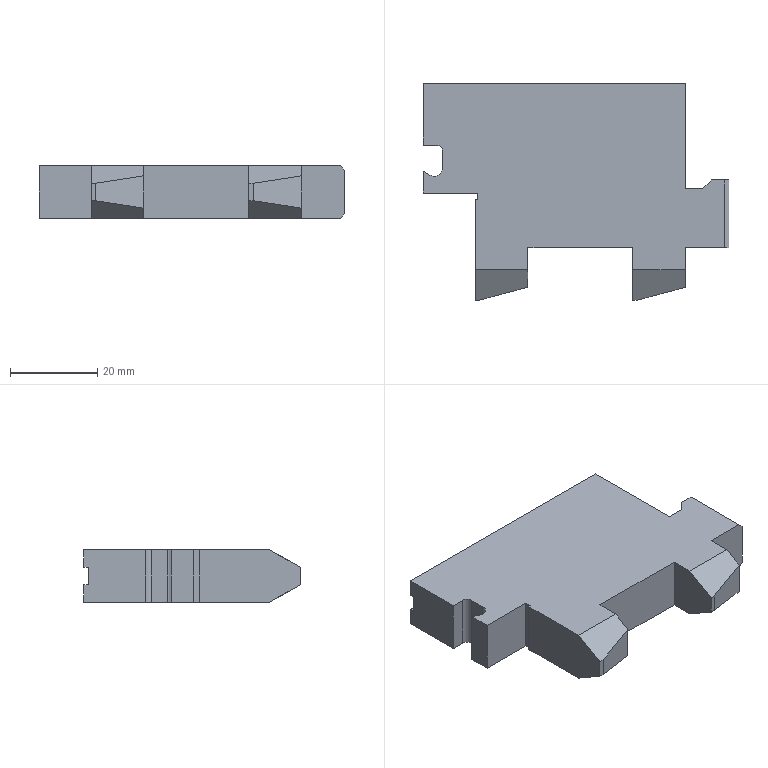Part | SolidWorks | features ICE 2, Chamfer 1, Extrusion 1 | 1 solid | 38 faces | box 70 x 49.5 x 12 mm | volume 28944 mm3 | plane 36 | cylinder 2 | commonest cylinder face diameters 3 x1 4 x1
STEP:
#1=CARTESIAN_POINT('',(0.,25.,-2.));
#2=VERTEX_POINT('',#1);
#3=CARTESIAN_POINT('',(0.,25.,-6.));
#4=VERTEX_POINT('',#3);
#5=CARTESIAN_POINT('',(0.,25.,6.));
#6=DIRECTION('',(0.,0.,-1.));
#7=VECTOR('',#6,1000.);
#8=LINE('',#5,#7);
#9=EDGE_CURVE('',#2,#4,#8,.T.);
#10=ORIENTED_EDGE('',*,*,#9,.F.);
#11=CARTESIAN_POINT('',(60.,25.,-2.));
#12=VERTEX_POINT('',#11);
#13=CARTESIAN_POINT('',(0.,25.,-2.));
#14=DIRECTION('',(-1.,0.,0.));
#15=VECTOR('',#14,1000.);
#16=LINE('',#13,#15);
#17=EDGE_CURVE('',#12,#2,#16,.T.);
#18=ORIENTED_EDGE('',*,*,#17,.F.);
#19=CARTESIAN_POINT('',(60.,25.,-6.));
#20=VERTEX_POINT('',#19);
#21=CARTESIAN_POINT('',(60.,25.,6.));
#22=DIRECTION('',(0.,0.,-1.));
#23=VECTOR('',#22,1000.);
#24=LINE('',#21,#23);
#25=EDGE_CURVE('',#12,#20,#24,.T.);
#26=ORIENTED_EDGE('',*,*,#25,.T.);
#27=CARTESIAN_POINT('',(0.,25.,-6.));
#28=DIRECTION('',(-1.,0.,0.));
#29=VECTOR('',#28,1000.);
#30=LINE('',#27,#29);
#31=EDGE_CURVE('',#20,#4,#30,.T.);
#32=ORIENTED_EDGE('',*,*,#31,.T.);
#33=EDGE_LOOP('',(#10,#18,#26,#32));
#34=FACE_OUTER_BOUND('',#33,.T.);
#35=CARTESIAN_POINT('',(0.,25.,6.));
#36=DIRECTION('',(0.,-1.,0.));
#37=DIRECTION('',(1.,0.,0.));
#38=AXIS2_PLACEMENT_3D('',#35,#36,#37);
#39=PLANE('',#38);
#40=ADVANCED_FACE('',(#34),#39,.F.);
#41=CARTESIAN_POINT('',(0.,0.,-6.));
#42=VERTEX_POINT('',#41);
#43=CARTESIAN_POINT('',(12.5,0.,-6.));
#44=VERTEX_POINT('',#43);
#45=CARTESIAN_POINT('',(12.5,0.,-6.));
#46=DIRECTION('',(1.,0.,0.));
#47=VECTOR('',#46,1000.);
#48=LINE('',#45,#47);
#49=EDGE_CURVE('',#42,#44,#48,.T.);
#50=ORIENTED_EDGE('',*,*,#49,.T.);
#51=CARTESIAN_POINT('',(12.5,0.,6.));
#52=VERTEX_POINT('',#51);
#53=CARTESIAN_POINT('',(12.5,0.,6.));
#54=DIRECTION('',(0.,0.,-1.));
#55=VECTOR('',#54,1000.);
#56=LINE('',#53,#55);
#57=EDGE_CURVE('',#52,#44,#56,.T.);
#58=ORIENTED_EDGE('',*,*,#57,.F.);
#59=CARTESIAN_POINT('',(0.,0.,6.));
#60=VERTEX_POINT('',#59);
#61=CARTESIAN_POINT('',(12.5,0.,6.));
#62=DIRECTION('',(1.,0.,0.));
#63=VECTOR('',#62,1000.);
#64=LINE('',#61,#63);
#65=EDGE_CURVE('',#60,#52,#64,.T.);
#66=ORIENTED_EDGE('',*,*,#65,.F.);
#67=CARTESIAN_POINT('',(0.,0.,6.));
#68=DIRECTION('',(0.,0.,-1.));
#69=VECTOR('',#68,1000.);
#70=LINE('',#67,#69);
#71=EDGE_CURVE('',#60,#42,#70,.T.);
#72=ORIENTED_EDGE('',*,*,#71,.T.);
#73=EDGE_LOOP('',(#50,#58,#66,#72));
#74=FACE_OUTER_BOUND('',#73,.T.);
#75=CARTESIAN_POINT('',(12.5,0.,6.));
#76=DIRECTION('',(0.,1.,0.));
#77=DIRECTION('',(-1.,0.,0.));
#78=AXIS2_PLACEMENT_3D('',#75,#76,#77);
#79=PLANE('',#78);
#80=ADVANCED_FACE('',(#74),#79,.F.);
#81=CARTESIAN_POINT('',(12.5,-1.5,-6.));
#82=VERTEX_POINT('',#81);
#83=CARTESIAN_POINT('',(12.5,0.,-6.));
#84=DIRECTION('',(0.,-1.,0.));
#85=VECTOR('',#84,1000.);
#86=LINE('',#83,#85);
#87=EDGE_CURVE('',#44,#82,#86,.T.);
#88=ORIENTED_EDGE('',*,*,#87,.T.);
#89=CARTESIAN_POINT('',(12.5,-1.5,6.));
#90=VERTEX_POINT('',#89);
#91=CARTESIAN_POINT('',(12.5,-1.5,6.));
#92=DIRECTION('',(0.,0.,-1.));
#93=VECTOR('',#92,1000.);
#94=LINE('',#91,#93);
#95=EDGE_CURVE('',#90,#82,#94,.T.);
#96=ORIENTED_EDGE('',*,*,#95,.F.);
#97=CARTESIAN_POINT('',(12.5,0.,6.));
#98=DIRECTION('',(0.,-1.,0.));
#99=VECTOR('',#98,1000.);
#100=LINE('',#97,#99);
#101=EDGE_CURVE('',#52,#90,#100,.T.);
#102=ORIENTED_EDGE('',*,*,#101,.F.);
#103=ORIENTED_EDGE('',*,*,#57,.T.);
#104=EDGE_LOOP('',(#88,#96,#102,#103));
#105=FACE_OUTER_BOUND('',#104,.T.);
#106=CARTESIAN_POINT('',(12.5,0.,6.));
#107=DIRECTION('',(1.,0.,0.));
#108=DIRECTION('',(0.,0.,-1.));
#109=AXIS2_PLACEMENT_3D('',#106,#107,#108);
#110=PLANE('',#109);
#111=ADVANCED_FACE('',(#105),#110,.F.);
#112=CARTESIAN_POINT('',(12.,-1.5,-6.));
#113=VERTEX_POINT('',#112);
#114=CARTESIAN_POINT('',(12.5,-1.5,-6.));
#115=DIRECTION('',(-1.,0.,0.));
#116=VECTOR('',#115,1000.);
#117=LINE('',#114,#116);
#118=EDGE_CURVE('',#82,#113,#117,.T.);
#119=ORIENTED_EDGE('',*,*,#118,.T.);
#120=CARTESIAN_POINT('',(12.,-1.5,6.));
#121=VERTEX_POINT('',#120);
#122=CARTESIAN_POINT('',(12.,-1.5,6.));
#123=DIRECTION('',(0.,0.,-1.));
#124=VECTOR('',#123,1000.);
#125=LINE('',#122,#124);
#126=EDGE_CURVE('',#121,#113,#125,.T.);
#127=ORIENTED_EDGE('',*,*,#126,.F.);
#128=CARTESIAN_POINT('',(12.5,-1.5,6.));
#129=DIRECTION('',(-1.,0.,0.));
#130=VECTOR('',#129,1000.);
#131=LINE('',#128,#130);
#132=EDGE_CURVE('',#90,#121,#131,.T.);
#133=ORIENTED_EDGE('',*,*,#132,.F.);
#134=ORIENTED_EDGE('',*,*,#95,.T.);
#135=EDGE_LOOP('',(#119,#127,#133,#134));
#136=FACE_OUTER_BOUND('',#135,.T.);
#137=CARTESIAN_POINT('',(12.5,-1.5,6.));
#138=DIRECTION('',(0.,-1.,0.));
#139=DIRECTION('',(0.,0.,-1.));
#140=AXIS2_PLACEMENT_3D('',#137,#138,#139);
#141=PLANE('',#140);
#142=ADVANCED_FACE('',(#136),#141,.F.);
#143=CARTESIAN_POINT('',(12.,-17.572,-6.));
#144=VERTEX_POINT('',#143);
#145=CARTESIAN_POINT('',(12.,-1.5,-6.));
#146=DIRECTION('',(0.,-1.,0.));
#147=VECTOR('',#146,1000.);
#148=LINE('',#145,#147);
#149=EDGE_CURVE('',#113,#144,#148,.T.);
#150=ORIENTED_EDGE('',*,*,#149,.T.);
#151=CARTESIAN_POINT('',(12.,-24.5,-2.));
#152=VERTEX_POINT('',#151);
#153=CARTESIAN_POINT('',(12.,-24.5,-2.));
#154=DIRECTION('',(0.,0.866,-0.5));
#155=VECTOR('',#154,1000.);
#156=LINE('',#153,#155);
#157=EDGE_CURVE('',#152,#144,#156,.T.);
#158=ORIENTED_EDGE('',*,*,#157,.F.);
#159=CARTESIAN_POINT('',(12.,-24.5,2.));
#160=VERTEX_POINT('',#159);
#161=CARTESIAN_POINT('',(12.,-24.5,6.));
#162=DIRECTION('',(0.,0.,-1.));
#163=VECTOR('',#162,1000.);
#164=LINE('',#161,#163);
#165=EDGE_CURVE('',#160,#152,#164,.T.);
#166=ORIENTED_EDGE('',*,*,#165,.F.);
#167=CARTESIAN_POINT('',(12.,-17.572,6.));
#168=VERTEX_POINT('',#167);
#169=CARTESIAN_POINT('',(12.,-24.5,2.));
#170=DIRECTION('',(0.,-0.866,-0.5));
#171=VECTOR('',#170,1000.);
#172=LINE('',#169,#171);
#173=EDGE_CURVE('',#168,#160,#172,.T.);
#174=ORIENTED_EDGE('',*,*,#173,.F.);
#175=CARTESIAN_POINT('',(12.,-1.5,6.));
#176=DIRECTION('',(0.,-1.,0.));
#177=VECTOR('',#176,1000.);
#178=LINE('',#175,#177);
#179=EDGE_CURVE('',#121,#168,#178,.T.);
#180=ORIENTED_EDGE('',*,*,#179,.F.);
#181=ORIENTED_EDGE('',*,*,#126,.T.);
#182=EDGE_LOOP('',(#150,#158,#166,#174,#180,#181));
#183=FACE_OUTER_BOUND('',#182,.T.);
#184=CARTESIAN_POINT('',(12.,-1.5,6.));
#185=DIRECTION('',(1.,0.,0.));
#186=DIRECTION('',(0.,1.,0.));
#187=AXIS2_PLACEMENT_3D('',#184,#185,#186);
#188=PLANE('',#187);
#189=ADVANCED_FACE('',(#183),#188,.F.);
#190=ORIENTED_EDGE('',*,*,#165,.T.);
#191=CARTESIAN_POINT('',(13.,-24.5,-2.));
#192=VERTEX_POINT('',#191);
#193=CARTESIAN_POINT('',(70.,-24.5,-2.));
#194=DIRECTION('',(-1.,0.,0.));
#195=VECTOR('',#194,1000.);
#196=LINE('',#193,#195);
#197=EDGE_CURVE('',#192,#152,#196,.T.);
#198=ORIENTED_EDGE('',*,*,#197,.F.);
#199=CARTESIAN_POINT('',(13.,-24.5,2.));
#200=VERTEX_POINT('',#199);
#201=CARTESIAN_POINT('',(13.,-24.5,6.));
#202=DIRECTION('',(0.,0.,-1.));
#203=VECTOR('',#202,1000.);
#204=LINE('',#201,#203);
#205=EDGE_CURVE('',#200,#192,#204,.T.);
#206=ORIENTED_EDGE('',*,*,#205,.F.);
#207=CARTESIAN_POINT('',(70.,-24.5,2.));
#208=DIRECTION('',(-1.,0.,0.));
#209=VECTOR('',#208,1000.);
#210=LINE('',#207,#209);
#211=EDGE_CURVE('',#200,#160,#210,.T.);
#212=ORIENTED_EDGE('',*,*,#211,.T.);
#213=EDGE_LOOP('',(#190,#198,#206,#212));
#214=FACE_OUTER_BOUND('',#213,.T.);
#215=CARTESIAN_POINT('',(13.,-24.5,6.));
#216=DIRECTION('',(0.,1.,0.));
#217=DIRECTION('',(0.,0.,1.));
#218=AXIS2_PLACEMENT_3D('',#215,#216,#217);
#219=PLANE('',#218);
#220=ADVANCED_FACE('',(#214),#219,.F.);
#221=ORIENTED_EDGE('',*,*,#205,.T.);
#222=CARTESIAN_POINT('',(24.,-21.553,-3.702));
#223=VERTEX_POINT('',#222);
#224=CARTESIAN_POINT('',(22.63,-21.92,-3.49));
#225=DIRECTION('',(0.9553,0.256,-0.1478));
#226=VECTOR('',#225,1000.);
#227=LINE('',#224,#226);
#228=EDGE_CURVE('',#192,#223,#227,.T.);
#229=ORIENTED_EDGE('',*,*,#228,.T.);
#230=CARTESIAN_POINT('',(24.,-21.553,3.702));
#231=VERTEX_POINT('',#230);
#232=CARTESIAN_POINT('',(24.,-21.553,6.));
#233=DIRECTION('',(0.,0.,-1.));
#234=VECTOR('',#233,1000.);
#235=LINE('',#232,#234);
#236=EDGE_CURVE('',#231,#223,#235,.T.);
#237=ORIENTED_EDGE('',*,*,#236,.F.);
#238=CARTESIAN_POINT('',(24.324,-21.466,3.752));
#239=DIRECTION('',(-0.9553,-0.256,-0.1478));
#240=VECTOR('',#239,1000.);
#241=LINE('',#238,#240);
#242=EDGE_CURVE('',#231,#200,#241,.T.);
#243=ORIENTED_EDGE('',*,*,#242,.T.);
#244=EDGE_LOOP('',(#221,#229,#237,#243));
#245=FACE_OUTER_BOUND('',#244,.T.);
#246=CARTESIAN_POINT('',(24.,-21.553,6.));
#247=DIRECTION('',(-0.2588,0.9659,0.));
#248=DIRECTION('',(-0.9659,-0.2588,0.));
#249=AXIS2_PLACEMENT_3D('',#246,#247,#248);
#250=PLANE('',#249);
#251=ADVANCED_FACE('',(#245),#250,.F.);
#252=ORIENTED_EDGE('',*,*,#236,.T.);
#253=CARTESIAN_POINT('',(24.,-17.572,-6.));
#254=VERTEX_POINT('',#253);
#255=CARTESIAN_POINT('',(24.,-18.964,-5.196));
#256=DIRECTION('',(0.,0.866,-0.5));
#257=VECTOR('',#256,1000.);
#258=LINE('',#255,#257);
#259=EDGE_CURVE('',#223,#254,#258,.T.);
#260=ORIENTED_EDGE('',*,*,#259,.T.);
#261=CARTESIAN_POINT('',(24.,-12.5,-6.));
#262=VERTEX_POINT('',#261);
#263=CARTESIAN_POINT('',(24.,-12.5,-6.));
#264=DIRECTION('',(0.,1.,0.));
#265=VECTOR('',#264,1000.);
#266=LINE('',#263,#265);
#267=EDGE_CURVE('',#254,#262,#266,.T.);
#268=ORIENTED_EDGE('',*,*,#267,.T.);
#269=CARTESIAN_POINT('',(24.,-12.5,6.));
#270=VERTEX_POINT('',#269);
#271=CARTESIAN_POINT('',(24.,-12.5,6.));
#272=DIRECTION('',(0.,0.,-1.));
#273=VECTOR('',#272,1000.);
#274=LINE('',#271,#273);
#275=EDGE_CURVE('',#270,#262,#274,.T.);
#276=ORIENTED_EDGE('',*,*,#275,.F.);
#277=CARTESIAN_POINT('',(24.,-17.572,6.));
#278=VERTEX_POINT('',#277);
#279=CARTESIAN_POINT('',(24.,-12.5,6.));
#280=DIRECTION('',(0.,1.,0.));
#281=VECTOR('',#280,1000.);
#282=LINE('',#279,#281);
#283=EDGE_CURVE('',#278,#270,#282,.T.);
#284=ORIENTED_EDGE('',*,*,#283,.F.);
#285=CARTESIAN_POINT('',(24.,-13.768,8.196));
#286=DIRECTION('',(0.,-0.866,-0.5));
#287=VECTOR('',#286,1000.);
#288=LINE('',#285,#287);
#289=EDGE_CURVE('',#278,#231,#288,.T.);
#290=ORIENTED_EDGE('',*,*,#289,.T.);
#291=EDGE_LOOP('',(#252,#260,#268,#276,#284,#290));
#292=FACE_OUTER_BOUND('',#291,.T.);
#293=CARTESIAN_POINT('',(24.,-12.5,6.));
#294=DIRECTION('',(-1.,0.,0.));
#295=DIRECTION('',(0.,0.,1.));
#296=AXIS2_PLACEMENT_3D('',#293,#294,#295);
#297=PLANE('',#296);
#298=ADVANCED_FACE('',(#292),#297,.F.);
#299=CARTESIAN_POINT('',(48.,-12.5,-6.));
#300=VERTEX_POINT('',#299);
#301=CARTESIAN_POINT('',(48.,-12.5,-6.));
#302=DIRECTION('',(1.,0.,0.));
#303=VECTOR('',#302,1000.);
#304=LINE('',#301,#303);
#305=EDGE_CURVE('',#262,#300,#304,.T.);
#306=ORIENTED_EDGE('',*,*,#305,.T.);
#307=CARTESIAN_POINT('',(48.,-12.5,6.));
#308=VERTEX_POINT('',#307);
#309=CARTESIAN_POINT('',(48.,-12.5,6.));
#310=DIRECTION('',(0.,0.,-1.));
#311=VECTOR('',#310,1000.);
#312=LINE('',#309,#311);
#313=EDGE_CURVE('',#308,#300,#312,.T.);
#314=ORIENTED_EDGE('',*,*,#313,.F.);
#315=CARTESIAN_POINT('',(48.,-12.5,6.));
#316=DIRECTION('',(1.,0.,0.));
#317=VECTOR('',#316,1000.);
#318=LINE('',#315,#317);
#319=EDGE_CURVE('',#270,#308,#318,.T.);
#320=ORIENTED_EDGE('',*,*,#319,.F.);
#321=ORIENTED_EDGE('',*,*,#275,.T.);
#322=EDGE_LOOP('',(#306,#314,#320,#321));
#323=FACE_OUTER_BOUND('',#322,.T.);
#324=CARTESIAN_POINT('',(48.,-12.5,6.));
#325=DIRECTION('',(0.,1.,0.));
#326=DIRECTION('',(-1.,0.,0.));
#327=AXIS2_PLACEMENT_3D('',#324,#325,#326);
#328=PLANE('',#327);
#329=ADVANCED_FACE('',(#323),#328,.F.);
#330=CARTESIAN_POINT('',(48.,-17.572,-6.));
#331=VERTEX_POINT('',#330);
#332=CARTESIAN_POINT('',(48.,-24.5,-6.));
#333=DIRECTION('',(0.,-1.,0.));
#334=VECTOR('',#333,1000.);
#335=LINE('',#332,#334);
#336=EDGE_CURVE('',#300,#331,#335,.T.);
#337=ORIENTED_EDGE('',*,*,#336,.T.);
#338=CARTESIAN_POINT('',(48.,-24.5,-2.));
#339=VERTEX_POINT('',#338);
#340=CARTESIAN_POINT('',(48.,-27.964,0.));
#341=DIRECTION('',(0.,-0.866,0.5));
#342=VECTOR('',#341,1000.);
#343=LINE('',#340,#342);
#344=EDGE_CURVE('',#331,#339,#343,.T.);
#345=ORIENTED_EDGE('',*,*,#344,.T.);
#346=CARTESIAN_POINT('',(48.,-24.5,2.));
#347=VERTEX_POINT('',#346);
#348=CARTESIAN_POINT('',(48.,-24.5,6.));
#349=DIRECTION('',(0.,0.,-1.));
#350=VECTOR('',#349,1000.);
#351=LINE('',#348,#350);
#352=EDGE_CURVE('',#347,#339,#351,.T.);
#353=ORIENTED_EDGE('',*,*,#352,.F.);
#354=CARTESIAN_POINT('',(48.,-17.572,6.));
#355=VERTEX_POINT('',#354);
#356=CARTESIAN_POINT('',(48.,-22.768,3.));
#357=DIRECTION('',(0.,0.866,0.5));
#358=VECTOR('',#357,1000.);
#359=LINE('',#356,#358);
#360=EDGE_CURVE('',#347,#355,#359,.T.);
#361=ORIENTED_EDGE('',*,*,#360,.T.);
#362=CARTESIAN_POINT('',(48.,-24.5,6.));
#363=DIRECTION('',(0.,-1.,0.));
#364=VECTOR('',#363,1000.);
#365=LINE('',#362,#364);
#366=EDGE_CURVE('',#308,#355,#365,.T.);
#367=ORIENTED_EDGE('',*,*,#366,.F.);
#368=ORIENTED_EDGE('',*,*,#313,.T.);
#369=EDGE_LOOP('',(#337,#345,#353,#361,#367,#368));
#370=FACE_OUTER_BOUND('',#369,.T.);
#371=CARTESIAN_POINT('',(48.,-24.5,6.));
#372=DIRECTION('',(1.,0.,0.));
#373=DIRECTION('',(0.,0.,-1.));
#374=AXIS2_PLACEMENT_3D('',#371,#372,#373);
#375=PLANE('',#374);
#376=ADVANCED_FACE('',(#370),#375,.F.);
#377=ORIENTED_EDGE('',*,*,#352,.T.);
#378=CARTESIAN_POINT('',(49.,-24.5,-2.));
#379=VERTEX_POINT('',#378);
#380=CARTESIAN_POINT('',(70.,-24.5,-2.));
#381=DIRECTION('',(-1.,0.,0.));
#382=VECTOR('',#381,1000.);
#383=LINE('',#380,#382);
#384=EDGE_CURVE('',#379,#339,#383,.T.);
#385=ORIENTED_EDGE('',*,*,#384,.F.);
#386=CARTESIAN_POINT('',(49.,-24.5,2.));
#387=VERTEX_POINT('',#386);
#388=CARTESIAN_POINT('',(49.,-24.5,6.));
#389=DIRECTION('',(0.,0.,-1.));
#390=VECTOR('',#389,1000.);
#391=LINE('',#388,#390);
#392=EDGE_CURVE('',#387,#379,#391,.T.);
#393=ORIENTED_EDGE('',*,*,#392,.F.);
#394=CARTESIAN_POINT('',(70.,-24.5,2.));
#395=DIRECTION('',(-1.,0.,0.));
#396=VECTOR('',#395,1000.);
#397=LINE('',#394,#396);
#398=EDGE_CURVE('',#387,#347,#397,.T.);
#399=ORIENTED_EDGE('',*,*,#398,.T.);
#400=EDGE_LOOP('',(#377,#385,#393,#399));
#401=FACE_OUTER_BOUND('',#400,.T.);
#402=CARTESIAN_POINT('',(49.,-24.5,6.));
#403=DIRECTION('',(0.,1.,0.));
#404=DIRECTION('',(0.,0.,1.));
#405=AXIS2_PLACEMENT_3D('',#402,#403,#404);
#406=PLANE('',#405);
#407=ADVANCED_FACE('',(#401),#406,.F.);
#408=ORIENTED_EDGE('',*,*,#392,.T.);
#409=CARTESIAN_POINT('',(60.,-21.553,-3.702));
#410=VERTEX_POINT('',#409);
#411=CARTESIAN_POINT('',(58.63,-21.92,-3.49));
#412=DIRECTION('',(0.9553,0.256,-0.1478));
#413=VECTOR('',#412,1000.);
#414=LINE('',#411,#413);
#415=EDGE_CURVE('',#379,#410,#414,.T.);
#416=ORIENTED_EDGE('',*,*,#415,.T.);
#417=CARTESIAN_POINT('',(60.,-21.553,3.702));
#418=VERTEX_POINT('',#417);
#419=CARTESIAN_POINT('',(60.,-21.553,6.));
#420=DIRECTION('',(0.,0.,-1.));
#421=VECTOR('',#420,1000.);
#422=LINE('',#419,#421);
#423=EDGE_CURVE('',#418,#410,#422,.T.);
#424=ORIENTED_EDGE('',*,*,#423,.F.);
#425=CARTESIAN_POINT('',(60.324,-21.466,3.752));
#426=DIRECTION('',(-0.9553,-0.256,-0.1478));
#427=VECTOR('',#426,1000.);
#428=LINE('',#425,#427);
#429=EDGE_CURVE('',#418,#387,#428,.T.);
#430=ORIENTED_EDGE('',*,*,#429,.T.);
#431=EDGE_LOOP('',(#408,#416,#424,#430));
#432=FACE_OUTER_BOUND('',#431,.T.);
#433=CARTESIAN_POINT('',(60.,-21.553,6.));
#434=DIRECTION('',(-0.2588,0.9659,0.));
#435=DIRECTION('',(-0.9659,-0.2588,0.));
#436=AXIS2_PLACEMENT_3D('',#433,#434,#435);
#437=PLANE('',#436);
#438=ADVANCED_FACE('',(#432),#437,.F.);
#439=ORIENTED_EDGE('',*,*,#423,.T.);
#440=CARTESIAN_POINT('',(60.,-17.572,-6.));
#441=VERTEX_POINT('',#440);
#442=CARTESIAN_POINT('',(60.,-25.754,-1.276));
#443=DIRECTION('',(0.,0.866,-0.5));
#444=VECTOR('',#443,1000.);
#445=LINE('',#442,#444);
#446=EDGE_CURVE('',#410,#441,#445,.T.);
#447=ORIENTED_EDGE('',*,*,#446,.T.);
#448=CARTESIAN_POINT('',(60.,-12.5,-6.));
#449=VERTEX_POINT('',#448);
#450=CARTESIAN_POINT('',(60.,-21.553,-6.));
#451=DIRECTION('',(0.,1.,0.));
#452=VECTOR('',#451,1000.);
#453=LINE('',#450,#452);
#454=EDGE_CURVE('',#441,#449,#453,.T.);
#455=ORIENTED_EDGE('',*,*,#454,.T.);
#456=CARTESIAN_POINT('',(60.,-12.5,6.));
#457=VERTEX_POINT('',#456);
#458=CARTESIAN_POINT('',(60.,-12.5,6.));
#459=DIRECTION('',(0.,0.,-1.));
#460=VECTOR('',#459,1000.);
#461=LINE('',#458,#460);
#462=EDGE_CURVE('',#457,#449,#461,.T.);
#463=ORIENTED_EDGE('',*,*,#462,.F.);
#464=CARTESIAN_POINT('',(60.,-17.572,6.));
#465=VERTEX_POINT('',#464);
#466=CARTESIAN_POINT('',(60.,-21.553,6.));
#467=DIRECTION('',(0.,1.,0.));
#468=VECTOR('',#467,1000.);
#469=LINE('',#466,#468);
#470=EDGE_CURVE('',#465,#457,#469,.T.);
#471=ORIENTED_EDGE('',*,*,#470,.F.);
#472=CARTESIAN_POINT('',(60.,-20.557,4.276));
#473=DIRECTION('',(0.,-0.866,-0.5));
#474=VECTOR('',#473,1000.);
#475=LINE('',#472,#474);
#476=EDGE_CURVE('',#465,#418,#475,.T.);
#477=ORIENTED_EDGE('',*,*,#476,.T.);
#478=EDGE_LOOP('',(#439,#447,#455,#463,#471,#477));
#479=FACE_OUTER_BOUND('',#478,.T.);
#480=CARTESIAN_POINT('',(60.,-21.553,6.));
#481=DIRECTION('',(-1.,0.,0.));
#482=DIRECTION('',(0.,-1.,0.));
#483=AXIS2_PLACEMENT_3D('',#480,#481,#482);
#484=PLANE('',#483);
#485=ADVANCED_FACE('',(#479),#484,.F.);
#486=CARTESIAN_POINT('',(69.,-12.5,-6.));
#487=VERTEX_POINT('',#486);
#488=CARTESIAN_POINT('',(70.,-12.5,-6.));
#489=DIRECTION('',(1.,0.,0.));
#490=VECTOR('',#489,1000.);
#491=LINE('',#488,#490);
#492=EDGE_CURVE('',#449,#487,#491,.T.);
#493=ORIENTED_EDGE('',*,*,#492,.T.);
#494=CARTESIAN_POINT('',(70.,-12.5,-5.));
#495=VERTEX_POINT('',#494);
#496=CARTESIAN_POINT('',(70.,-12.5,-5.));
#497=DIRECTION('',(0.7071,0.,0.7071));
#498=VECTOR('',#497,1000.);
#499=LINE('',#496,#498);
#500=EDGE_CURVE('',#487,#495,#499,.T.);
#501=ORIENTED_EDGE('',*,*,#500,.T.);
#502=CARTESIAN_POINT('',(70.,-12.5,5.));
#503=VERTEX_POINT('',#502);
#504=CARTESIAN_POINT('',(70.,-12.5,6.));
#505=DIRECTION('',(0.,0.,-1.));
#506=VECTOR('',#505,1000.);
#507=LINE('',#504,#506);
#508=EDGE_CURVE('',#503,#495,#507,.T.);
#509=ORIENTED_EDGE('',*,*,#508,.F.);
#510=CARTESIAN_POINT('',(69.,-12.5,6.));
#511=VERTEX_POINT('',#510);
#512=CARTESIAN_POINT('',(69.,-12.5,6.));
#513=DIRECTION('',(-0.7071,0.,0.7071));
#514=VECTOR('',#513,1000.);
#515=LINE('',#512,#514);
#516=EDGE_CURVE('',#503,#511,#515,.T.);
#517=ORIENTED_EDGE('',*,*,#516,.T.);
#518=CARTESIAN_POINT('',(70.,-12.5,6.));
#519=DIRECTION('',(1.,0.,0.));
#520=VECTOR('',#519,1000.);
#521=LINE('',#518,#520);
#522=EDGE_CURVE('',#457,#511,#521,.T.);
#523=ORIENTED_EDGE('',*,*,#522,.F.);
#524=ORIENTED_EDGE('',*,*,#462,.T.);
#525=EDGE_LOOP('',(#493,#501,#509,#517,#523,#524));
#526=FACE_OUTER_BOUND('',#525,.T.);
#527=CARTESIAN_POINT('',(70.,-12.5,6.));
#528=DIRECTION('',(0.,1.,0.));
#529=DIRECTION('',(-1.,0.,0.));
#530=AXIS2_PLACEMENT_3D('',#527,#528,#529);
#531=PLANE('',#530);
#532=ADVANCED_FACE('',(#526),#531,.F.);
#533=ORIENTED_EDGE('',*,*,#508,.T.);
#534=CARTESIAN_POINT('',(70.,3.,-5.));
#535=VERTEX_POINT('',#534);
#536=CARTESIAN_POINT('',(70.,3.,-5.));
#537=DIRECTION('',(0.,1.,0.));
#538=VECTOR('',#537,1000.);
#539=LINE('',#536,#538);
#540=EDGE_CURVE('',#495,#535,#539,.T.);
#541=ORIENTED_EDGE('',*,*,#540,.T.);
#542=CARTESIAN_POINT('',(70.,3.,5.));
#543=VERTEX_POINT('',#542);
#544=CARTESIAN_POINT('',(70.,3.,6.));
#545=DIRECTION('',(0.,0.,-1.));
#546=VECTOR('',#545,1000.);
#547=LINE('',#544,#546);
#548=EDGE_CURVE('',#543,#535,#547,.T.);
#549=ORIENTED_EDGE('',*,*,#548,.F.);
#550=CARTESIAN_POINT('',(70.,-12.5,5.));
#551=DIRECTION('',(0.,-1.,0.));
#552=VECTOR('',#551,1000.);
#553=LINE('',#550,#552);
#554=EDGE_CURVE('',#543,#503,#553,.T.);
#555=ORIENTED_EDGE('',*,*,#554,.T.);
#556=EDGE_LOOP('',(#533,#541,#549,#555));
#557=FACE_OUTER_BOUND('',#556,.T.);
#558=CARTESIAN_POINT('',(70.,3.,6.));
#559=DIRECTION('',(-1.,0.,0.));
#560=DIRECTION('',(0.,0.,1.));
#561=AXIS2_PLACEMENT_3D('',#558,#559,#560);
#562=PLANE('',#561);
#563=ADVANCED_FACE('',(#557),#562,.F.);
#564=ORIENTED_EDGE('',*,*,#548,.T.);
#565=CARTESIAN_POINT('',(69.,3.,-6.));
#566=VERTEX_POINT('',#565);
#567=CARTESIAN_POINT('',(70.,3.,-5.));
#568=DIRECTION('',(-0.7071,0.,-0.7071));
#569=VECTOR('',#568,1000.);
#570=LINE('',#567,#569);
#571=EDGE_CURVE('',#535,#566,#570,.T.);
#572=ORIENTED_EDGE('',*,*,#571,.T.);
#573=CARTESIAN_POINT('',(66.,3.,-6.));
#574=VERTEX_POINT('',#573);
#575=CARTESIAN_POINT('',(66.,3.,-6.));
#576=DIRECTION('',(-1.,0.,0.));
#577=VECTOR('',#576,1000.);
#578=LINE('',#575,#577);
#579=EDGE_CURVE('',#566,#574,#578,.T.);
#580=ORIENTED_EDGE('',*,*,#579,.T.);
#581=CARTESIAN_POINT('',(66.,3.,6.));
#582=VERTEX_POINT('',#581);
#583=CARTESIAN_POINT('',(66.,3.,6.));
#584=DIRECTION('',(0.,0.,-1.));
#585=VECTOR('',#584,1000.);
#586=LINE('',#583,#585);
#587=EDGE_CURVE('',#582,#574,#586,.T.);
#588=ORIENTED_EDGE('',*,*,#587,.F.);
#589=CARTESIAN_POINT('',(69.,3.,6.));
#590=VERTEX_POINT('',#589);
#591=CARTESIAN_POINT('',(66.,3.,6.));
#592=DIRECTION('',(-1.,0.,0.));
#593=VECTOR('',#592,1000.);
#594=LINE('',#591,#593);
#595=EDGE_CURVE('',#590,#582,#594,.T.);
#596=ORIENTED_EDGE('',*,*,#595,.F.);
#597=CARTESIAN_POINT('',(69.,3.,6.));
#598=DIRECTION('',(0.7071,0.,-0.7071));
#599=VECTOR('',#598,1000.);
#600=LINE('',#597,#599);
#601=EDGE_CURVE('',#590,#543,#600,.T.);
#602=ORIENTED_EDGE('',*,*,#601,.T.);
#603=EDGE_LOOP('',(#564,#572,#580,#588,#596,#602));
#604=FACE_OUTER_BOUND('',#603,.T.);
#605=CARTESIAN_POINT('',(66.,3.,6.));
#606=DIRECTION('',(0.,-1.,0.));
#607=DIRECTION('',(1.,0.,0.));
#608=AXIS2_PLACEMENT_3D('',#605,#606,#607);
#609=PLANE('',#608);
#610=ADVANCED_FACE('',(#604),#609,.F.);
#611=CARTESIAN_POINT('',(64.,1.,-6.));
#612=VERTEX_POINT('',#611);
#613=CARTESIAN_POINT('',(64.,1.,-6.));
#614=DIRECTION('',(-0.7071,-0.7071,0.));
#615=VECTOR('',#614,1000.);
#616=LINE('',#613,#615);
#617=EDGE_CURVE('',#574,#612,#616,.T.);
#618=ORIENTED_EDGE('',*,*,#617,.T.);
#619=CARTESIAN_POINT('',(64.,1.,6.));
#620=VERTEX_POINT('',#619);
#621=CARTESIAN_POINT('',(64.,1.,6.));
#622=DIRECTION('',(0.,0.,-1.));
#623=VECTOR('',#622,1000.);
#624=LINE('',#621,#623);
#625=EDGE_CURVE('',#620,#612,#624,.T.);
#626=ORIENTED_EDGE('',*,*,#625,.F.);
#627=CARTESIAN_POINT('',(64.,1.,6.));
#628=DIRECTION('',(-0.7071,-0.7071,0.));
#629=VECTOR('',#628,1000.);
#630=LINE('',#627,#629);
#631=EDGE_CURVE('',#582,#620,#630,.T.);
#632=ORIENTED_EDGE('',*,*,#631,.F.);
#633=ORIENTED_EDGE('',*,*,#587,.T.);
#634=EDGE_LOOP('',(#618,#626,#632,#633));
#635=FACE_OUTER_BOUND('',#634,.T.);
#636=CARTESIAN_POINT('',(64.,1.,6.));
#637=DIRECTION('',(0.7071,-0.7071,0.));
#638=DIRECTION('',(0.7071,0.7071,0.));
#639=AXIS2_PLACEMENT_3D('',#636,#637,#638);
#640=PLANE('',#639);
#641=ADVANCED_FACE('',(#635),#640,.F.);
#642=CARTESIAN_POINT('',(60.,1.,-6.));
#643=VERTEX_POINT('',#642);
#644=CARTESIAN_POINT('',(60.,1.,-6.));
#645=DIRECTION('',(-1.,0.,0.));
#646=VECTOR('',#645,1000.);
#647=LINE('',#644,#646);
#648=EDGE_CURVE('',#612,#643,#647,.T.);
#649=ORIENTED_EDGE('',*,*,#648,.T.);
#650=CARTESIAN_POINT('',(60.,1.,6.));
#651=VERTEX_POINT('',#650);
#652=CARTESIAN_POINT('',(60.,1.,6.));
#653=DIRECTION('',(0.,0.,-1.));
#654=VECTOR('',#653,1000.);
#655=LINE('',#652,#654);
#656=EDGE_CURVE('',#651,#643,#655,.T.);
#657=ORIENTED_EDGE('',*,*,#656,.F.);
#658=CARTESIAN_POINT('',(60.,1.,6.));
#659=DIRECTION('',(-1.,0.,0.));
#660=VECTOR('',#659,1000.);
#661=LINE('',#658,#660);
#662=EDGE_CURVE('',#620,#651,#661,.T.);
#663=ORIENTED_EDGE('',*,*,#662,.F.);
#664=ORIENTED_EDGE('',*,*,#625,.T.);
#665=EDGE_LOOP('',(#649,#657,#663,#664));
#666=FACE_OUTER_BOUND('',#665,.T.);
#667=CARTESIAN_POINT('',(60.,1.,6.));
#668=DIRECTION('',(0.,-1.,0.));
#669=DIRECTION('',(1.,0.,0.));
#670=AXIS2_PLACEMENT_3D('',#667,#668,#669);
#671=PLANE('',#670);
#672=ADVANCED_FACE('',(#666),#671,.F.);
#673=ORIENTED_EDGE('',*,*,#25,.F.);
#674=CARTESIAN_POINT('',(60.,24.,-2.));
#675=VERTEX_POINT('',#674);
#676=CARTESIAN_POINT('',(60.,24.,-2.));
#677=DIRECTION('',(0.,1.,0.));
#678=VECTOR('',#677,1000.);
#679=LINE('',#676,#678);
#680=EDGE_CURVE('',#675,#12,#679,.T.);
#681=ORIENTED_EDGE('',*,*,#680,.F.);
#682=CARTESIAN_POINT('',(60.,24.,2.));
#683=VERTEX_POINT('',#682);
#684=CARTESIAN_POINT('',(60.,24.,-2.));
#685=DIRECTION('',(0.,0.,-1.));
#686=VECTOR('',#685,1000.);
#687=LINE('',#684,#686);
#688=EDGE_CURVE('',#683,#675,#687,.T.);
#689=ORIENTED_EDGE('',*,*,#688,.F.);
#690=CARTESIAN_POINT('',(60.,25.,2.));
#691=VERTEX_POINT('',#690);
#692=CARTESIAN_POINT('',(60.,24.,2.));
#693=DIRECTION('',(0.,1.,0.));
#694=VECTOR('',#693,1000.);
#695=LINE('',#692,#694);
#696=EDGE_CURVE('',#683,#691,#695,.T.);
#697=ORIENTED_EDGE('',*,*,#696,.T.);
#698=CARTESIAN_POINT('',(60.,25.,6.));
#699=VERTEX_POINT('',#698);
#700=CARTESIAN_POINT('',(60.,25.,6.));
#701=DIRECTION('',(0.,0.,-1.));
#702=VECTOR('',#701,1000.);
#703=LINE('',#700,#702);
#704=EDGE_CURVE('',#699,#691,#703,.T.);
#705=ORIENTED_EDGE('',*,*,#704,.F.);
#706=CARTESIAN_POINT('',(60.,25.,6.));
#707=DIRECTION('',(0.,1.,0.));
#708=VECTOR('',#707,1000.);
#709=LINE('',#706,#708);
#710=EDGE_CURVE('',#651,#699,#709,.T.);
#711=ORIENTED_EDGE('',*,*,#710,.F.);
#712=ORIENTED_EDGE('',*,*,#656,.T.);
#713=CARTESIAN_POINT('',(60.,25.,-6.));
#714=DIRECTION('',(0.,1.,0.));
#715=VECTOR('',#714,1000.);
#716=LINE('',#713,#715);
#717=EDGE_CURVE('',#643,#20,#716,.T.);
#718=ORIENTED_EDGE('',*,*,#717,.T.);
#719=EDGE_LOOP('',(#673,#681,#689,#697,#705,#711,#712,#718));
#720=FACE_OUTER_BOUND('',#719,.T.);
#721=CARTESIAN_POINT('',(60.,25.,6.));
#722=DIRECTION('',(-1.,0.,0.));
#723=DIRECTION('',(0.,0.,1.));
#724=AXIS2_PLACEMENT_3D('',#721,#722,#723);
#725=PLANE('',#724);
#726=ADVANCED_FACE('',(#720),#725,.F.);
#727=ORIENTED_EDGE('',*,*,#704,.T.);
#728=CARTESIAN_POINT('',(0.,25.,2.));
#729=VERTEX_POINT('',#728);
#730=CARTESIAN_POINT('',(0.,25.,2.));
#731=DIRECTION('',(1.,0.,0.));
#732=VECTOR('',#731,1000.);
#733=LINE('',#730,#732);
#734=EDGE_CURVE('',#729,#691,#733,.T.);
#735=ORIENTED_EDGE('',*,*,#734,.F.);
#736=CARTESIAN_POINT('',(0.,25.,6.));
#737=VERTEX_POINT('',#736);
#738=CARTESIAN_POINT('',(0.,25.,6.));
#739=DIRECTION('',(0.,0.,-1.));
#740=VECTOR('',#739,1000.);
#741=LINE('',#738,#740);
#742=EDGE_CURVE('',#737,#729,#741,.T.);
#743=ORIENTED_EDGE('',*,*,#742,.F.);
#744=CARTESIAN_POINT('',(0.,25.,6.));
#745=DIRECTION('',(-1.,0.,0.));
#746=VECTOR('',#745,1000.);
#747=LINE('',#744,#746);
#748=EDGE_CURVE('',#699,#737,#747,.T.);
#749=ORIENTED_EDGE('',*,*,#748,.F.);
#750=EDGE_LOOP('',(#727,#735,#743,#749));
#751=FACE_OUTER_BOUND('',#750,.T.);
#752=CARTESIAN_POINT('',(0.,25.,6.));
#753=DIRECTION('',(0.,-1.,0.));
#754=DIRECTION('',(1.,0.,0.));
#755=AXIS2_PLACEMENT_3D('',#752,#753,#754);
#756=PLANE('',#755);
#757=ADVANCED_FACE('',(#751),#756,.F.);
#758=CARTESIAN_POINT('',(0.,24.,-2.));
#759=VERTEX_POINT('',#758);
#760=CARTESIAN_POINT('',(0.,24.,2.));
#761=VERTEX_POINT('',#760);
#762=CARTESIAN_POINT('',(0.,24.,-2.));
#763=DIRECTION('',(0.,0.,1.));
#764=VECTOR('',#763,1000.);
#765=LINE('',#762,#764);
#766=EDGE_CURVE('',#759,#761,#765,.T.);
#767=ORIENTED_EDGE('',*,*,#766,.F.);
#768=CARTESIAN_POINT('',(0.,24.,-2.));
#769=DIRECTION('',(0.,1.,0.));
#770=VECTOR('',#769,1000.);
#771=LINE('',#768,#770);
#772=EDGE_CURVE('',#759,#2,#771,.T.);
#773=ORIENTED_EDGE('',*,*,#772,.T.);
#774=ORIENTED_EDGE('',*,*,#9,.T.);
#775=CARTESIAN_POINT('',(0.,11.,-6.));
#776=VERTEX_POINT('',#775);
#777=CARTESIAN_POINT('',(0.,11.,-6.));
#778=DIRECTION('',(0.,-1.,0.));
#779=VECTOR('',#778,1000.);
#780=LINE('',#777,#779);
#781=EDGE_CURVE('',#4,#776,#780,.T.);
#782=ORIENTED_EDGE('',*,*,#781,.T.);
#783=CARTESIAN_POINT('',(0.,11.,6.));
#784=VERTEX_POINT('',#783);
#785=CARTESIAN_POINT('',(0.,11.,6.));
#786=DIRECTION('',(0.,0.,-1.));
#787=VECTOR('',#786,1000.);
#788=LINE('',#785,#787);
#789=EDGE_CURVE('',#784,#776,#788,.T.);
#790=ORIENTED_EDGE('',*,*,#789,.F.);
#791=CARTESIAN_POINT('',(0.,11.,6.));
#792=DIRECTION('',(0.,-1.,0.));
#793=VECTOR('',#792,1000.);
#794=LINE('',#791,#793);
#795=EDGE_CURVE('',#737,#784,#794,.T.);
#796=ORIENTED_EDGE('',*,*,#795,.F.);
#797=ORIENTED_EDGE('',*,*,#742,.T.);
#798=CARTESIAN_POINT('',(0.,24.,2.));
#799=DIRECTION('',(0.,1.,0.));
#800=VECTOR('',#799,1000.);
#801=LINE('',#798,#800);
#802=EDGE_CURVE('',#761,#729,#801,.T.);
#803=ORIENTED_EDGE('',*,*,#802,.F.);
#804=EDGE_LOOP('',(#767,#773,#774,#782,#790,#796,#797,#803));
#805=FACE_OUTER_BOUND('',#804,.T.);
#806=CARTESIAN_POINT('',(0.,11.,6.));
#807=DIRECTION('',(1.,0.,0.));
#808=DIRECTION('',(0.,0.,-1.));
#809=AXIS2_PLACEMENT_3D('',#806,#807,#808);
#810=PLANE('',#809);
#811=ADVANCED_FACE('',(#805),#810,.F.);
#812=CARTESIAN_POINT('',(3.,11.,-6.));
#813=VERTEX_POINT('',#812);
#814=CARTESIAN_POINT('',(3.,11.,-6.));
#815=DIRECTION('',(1.,0.,0.));
#816=VECTOR('',#815,1000.);
#817=LINE('',#814,#816);
#818=EDGE_CURVE('',#776,#813,#817,.T.);
#819=ORIENTED_EDGE('',*,*,#818,.T.);
#820=CARTESIAN_POINT('',(3.,11.,6.));
#821=VERTEX_POINT('',#820);
#822=CARTESIAN_POINT('',(3.,11.,6.));
#823=DIRECTION('',(0.,0.,-1.));
#824=VECTOR('',#823,1000.);
#825=LINE('',#822,#824);
#826=EDGE_CURVE('',#821,#813,#825,.T.);
#827=ORIENTED_EDGE('',*,*,#826,.F.);
#828=CARTESIAN_POINT('',(3.,11.,6.));
#829=DIRECTION('',(1.,0.,0.));
#830=VECTOR('',#829,1000.);
#831=LINE('',#828,#830);
#832=EDGE_CURVE('',#784,#821,#831,.T.);
#833=ORIENTED_EDGE('',*,*,#832,.F.);
#834=ORIENTED_EDGE('',*,*,#789,.T.);
#835=EDGE_LOOP('',(#819,#827,#833,#834));
#836=FACE_OUTER_BOUND('',#835,.T.);
#837=CARTESIAN_POINT('',(3.,11.,6.));
#838=DIRECTION('',(0.,1.,0.));
#839=DIRECTION('',(-1.,0.,0.));
#840=AXIS2_PLACEMENT_3D('',#837,#838,#839);
#841=PLANE('',#840);
#842=ADVANCED_FACE('',(#836),#841,.F.);
#843=CARTESIAN_POINT('',(4.5,9.5,-6.));
#844=VERTEX_POINT('',#843);
#845=CARTESIAN_POINT('',(3.,9.5,-6.));
#846=DIRECTION('',(0.,0.,-1.));
#847=DIRECTION('',(1.,0.,0.));
#848=AXIS2_PLACEMENT_3D('',#845,#846,#847);
#849=CIRCLE('',#848,1.5);
#850=EDGE_CURVE('',#813,#844,#849,.T.);
#851=ORIENTED_EDGE('',*,*,#850,.T.);
#852=CARTESIAN_POINT('',(4.5,9.5,6.));
#853=VERTEX_POINT('',#852);
#854=CARTESIAN_POINT('',(4.5,9.5,6.));
#855=DIRECTION('',(0.,0.,-1.));
#856=VECTOR('',#855,1000.);
#857=LINE('',#854,#856);
#858=EDGE_CURVE('',#853,#844,#857,.T.);
#859=ORIENTED_EDGE('',*,*,#858,.F.);
#860=CARTESIAN_POINT('',(3.,9.5,6.));
#861=DIRECTION('',(0.,0.,-1.));
#862=DIRECTION('',(1.,0.,0.));
#863=AXIS2_PLACEMENT_3D('',#860,#861,#862);
#864=CIRCLE('',#863,1.5);
#865=EDGE_CURVE('',#821,#853,#864,.T.);
#866=ORIENTED_EDGE('',*,*,#865,.F.);
#867=ORIENTED_EDGE('',*,*,#826,.T.);
#868=EDGE_LOOP('',(#851,#859,#866,#867));
#869=FACE_OUTER_BOUND('',#868,.T.);
#870=CARTESIAN_POINT('',(3.,9.5,6.));
#871=DIRECTION('',(0.,0.,-1.));
#872=DIRECTION('',(-1.,0.,0.));
#873=AXIS2_PLACEMENT_3D('',#870,#871,#872);
#874=CYLINDRICAL_SURFACE('',#873,1.5);
#875=ADVANCED_FACE('',(#869),#874,.F.);
#876=CARTESIAN_POINT('',(4.5,5.866,-6.));
#877=VERTEX_POINT('',#876);
#878=CARTESIAN_POINT('',(4.5,5.866,-6.));
#879=DIRECTION('',(0.,-1.,0.));
#880=VECTOR('',#879,1000.);
#881=LINE('',#878,#880);
#882=EDGE_CURVE('',#844,#877,#881,.T.);
#883=ORIENTED_EDGE('',*,*,#882,.T.);
#884=CARTESIAN_POINT('',(4.5,5.866,6.));
#885=VERTEX_POINT('',#884);
#886=CARTESIAN_POINT('',(4.5,5.866,6.));
#887=DIRECTION('',(0.,0.,-1.));
#888=VECTOR('',#887,1000.);
#889=LINE('',#886,#888);
#890=EDGE_CURVE('',#885,#877,#889,.T.);
#891=ORIENTED_EDGE('',*,*,#890,.F.);
#892=CARTESIAN_POINT('',(4.5,5.866,6.));
#893=DIRECTION('',(0.,-1.,0.));
#894=VECTOR('',#893,1000.);
#895=LINE('',#892,#894);
#896=EDGE_CURVE('',#853,#885,#895,.T.);
#897=ORIENTED_EDGE('',*,*,#896,.F.);
#898=ORIENTED_EDGE('',*,*,#858,.T.);
#899=EDGE_LOOP('',(#883,#891,#897,#898));
#900=FACE_OUTER_BOUND('',#899,.T.);
#901=CARTESIAN_POINT('',(4.5,5.866,6.));
#902=DIRECTION('',(1.,0.,0.));
#903=DIRECTION('',(0.,1.,0.));
#904=AXIS2_PLACEMENT_3D('',#901,#902,#903);
#905=PLANE('',#904);
#906=ADVANCED_FACE('',(#900),#905,.F.);
#907=CARTESIAN_POINT('',(1.5,4.134,-6.));
#908=VERTEX_POINT('',#907);
#909=CARTESIAN_POINT('',(2.5,5.866,-6.));
#910=DIRECTION('',(0.,0.,-1.));
#911=DIRECTION('',(1.,0.,0.));
#912=AXIS2_PLACEMENT_3D('',#909,#910,#911);
#913=CIRCLE('',#912,2.);
#914=EDGE_CURVE('',#877,#908,#913,.T.);
#915=ORIENTED_EDGE('',*,*,#914,.T.);
#916=CARTESIAN_POINT('',(1.5,4.134,6.));
#917=VERTEX_POINT('',#916);
#918=CARTESIAN_POINT('',(1.5,4.134,6.));
#919=DIRECTION('',(0.,0.,-1.));
#920=VECTOR('',#919,1000.);
#921=LINE('',#918,#920);
#922=EDGE_CURVE('',#917,#908,#921,.T.);
#923=ORIENTED_EDGE('',*,*,#922,.F.);
#924=CARTESIAN_POINT('',(2.5,5.866,6.));
#925=DIRECTION('',(0.,0.,-1.));
#926=DIRECTION('',(1.,0.,0.));
#927=AXIS2_PLACEMENT_3D('',#924,#925,#926);
#928=CIRCLE('',#927,2.);
#929=EDGE_CURVE('',#885,#917,#928,.T.);
#930=ORIENTED_EDGE('',*,*,#929,.F.);
#931=ORIENTED_EDGE('',*,*,#890,.T.);
#932=EDGE_LOOP('',(#915,#923,#930,#931));
#933=FACE_OUTER_BOUND('',#932,.T.);
#934=CARTESIAN_POINT('',(2.5,5.866,6.));
#935=DIRECTION('',(0.,0.,-1.));
#936=DIRECTION('',(-1.,0.,0.));
#937=AXIS2_PLACEMENT_3D('',#934,#935,#936);
#938=CYLINDRICAL_SURFACE('',#937,2.);
#939=ADVANCED_FACE('',(#933),#938,.F.);
#940=CARTESIAN_POINT('',(0.,5.,-6.));
#941=VERTEX_POINT('',#940);
#942=CARTESIAN_POINT('',(1.5,4.134,-6.));
#943=DIRECTION('',(-0.866,0.5,0.));
#944=VECTOR('',#943,1000.);
#945=LINE('',#942,#944);
#946=EDGE_CURVE('',#908,#941,#945,.T.);
#947=ORIENTED_EDGE('',*,*,#946,.T.);
#948=CARTESIAN_POINT('',(0.,5.,6.));
#949=VERTEX_POINT('',#948);
#950=CARTESIAN_POINT('',(0.,5.,6.));
#951=DIRECTION('',(0.,0.,-1.));
#952=VECTOR('',#951,1000.);
#953=LINE('',#950,#952);
#954=EDGE_CURVE('',#949,#941,#953,.T.);
#955=ORIENTED_EDGE('',*,*,#954,.F.);
#956=CARTESIAN_POINT('',(1.5,4.134,6.));
#957=DIRECTION('',(-0.866,0.5,0.));
#958=VECTOR('',#957,1000.);
#959=LINE('',#956,#958);
#960=EDGE_CURVE('',#917,#949,#959,.T.);
#961=ORIENTED_EDGE('',*,*,#960,.F.);
#962=ORIENTED_EDGE('',*,*,#922,.T.);
#963=EDGE_LOOP('',(#947,#955,#961,#962));
#964=FACE_OUTER_BOUND('',#963,.T.);
#965=CARTESIAN_POINT('',(1.5,4.134,6.));
#966=DIRECTION('',(-0.5,-0.866,0.));
#967=DIRECTION('',(0.866,-0.5,0.));
#968=AXIS2_PLACEMENT_3D('',#965,#966,#967);
#969=PLANE('',#968);
#970=ADVANCED_FACE('',(#964),#969,.F.);
#971=CARTESIAN_POINT('',(0.,0.,-6.));
#972=DIRECTION('',(0.,-1.,0.));
#973=VECTOR('',#972,1000.);
#974=LINE('',#971,#973);
#975=EDGE_CURVE('',#941,#42,#974,.T.);
#976=ORIENTED_EDGE('',*,*,#975,.T.);
#977=ORIENTED_EDGE('',*,*,#71,.F.);
#978=CARTESIAN_POINT('',(0.,0.,6.));
#979=DIRECTION('',(0.,-1.,0.));
#980=VECTOR('',#979,1000.);
#981=LINE('',#978,#980);
#982=EDGE_CURVE('',#949,#60,#981,.T.);
#983=ORIENTED_EDGE('',*,*,#982,.F.);
#984=ORIENTED_EDGE('',*,*,#954,.T.);
#985=EDGE_LOOP('',(#976,#977,#983,#984));
#986=FACE_OUTER_BOUND('',#985,.T.);
#987=CARTESIAN_POINT('',(0.,0.,6.));
#988=DIRECTION('',(1.,0.,0.));
#989=DIRECTION('',(0.,0.,-1.));
#990=AXIS2_PLACEMENT_3D('',#987,#988,#989);
#991=PLANE('',#990);
#992=ADVANCED_FACE('',(#986),#991,.F.);
#993=ORIENTED_EDGE('',*,*,#522,.T.);
#994=CARTESIAN_POINT('',(69.,3.,6.));
#995=DIRECTION('',(0.,1.,0.));
#996=VECTOR('',#995,1000.);
#997=LINE('',#994,#996);
#998=EDGE_CURVE('',#511,#590,#997,.T.);
#999=ORIENTED_EDGE('',*,*,#998,.T.);
#1000=ORIENTED_EDGE('',*,*,#595,.T.);
#1001=ORIENTED_EDGE('',*,*,#631,.T.);
#1002=ORIENTED_EDGE('',*,*,#662,.T.);
#1003=ORIENTED_EDGE('',*,*,#710,.T.);
#1004=ORIENTED_EDGE('',*,*,#748,.T.);
#1005=ORIENTED_EDGE('',*,*,#795,.T.);
#1006=ORIENTED_EDGE('',*,*,#832,.T.);
#1007=ORIENTED_EDGE('',*,*,#865,.T.);
#1008=ORIENTED_EDGE('',*,*,#896,.T.);
#1009=ORIENTED_EDGE('',*,*,#929,.T.);
#1010=ORIENTED_EDGE('',*,*,#960,.T.);
#1011=ORIENTED_EDGE('',*,*,#982,.T.);
#1012=ORIENTED_EDGE('',*,*,#65,.T.);
#1013=ORIENTED_EDGE('',*,*,#101,.T.);
#1014=ORIENTED_EDGE('',*,*,#132,.T.);
#1015=ORIENTED_EDGE('',*,*,#179,.T.);
#1016=CARTESIAN_POINT('',(2.5,-17.572,6.));
#1017=DIRECTION('',(-1.,0.,0.));
#1018=VECTOR('',#1017,1000.);
#1019=LINE('',#1016,#1018);
#1020=EDGE_CURVE('',#278,#168,#1019,.T.);
#1021=ORIENTED_EDGE('',*,*,#1020,.F.);
#1022=ORIENTED_EDGE('',*,*,#283,.T.);
#1023=ORIENTED_EDGE('',*,*,#319,.T.);
#1024=ORIENTED_EDGE('',*,*,#366,.T.);
#1025=CARTESIAN_POINT('',(2.5,-17.572,6.));
#1026=DIRECTION('',(-1.,0.,0.));
#1027=VECTOR('',#1026,1000.);
#1028=LINE('',#1025,#1027);
#1029=EDGE_CURVE('',#465,#355,#1028,.T.);
#1030=ORIENTED_EDGE('',*,*,#1029,.F.);
#1031=ORIENTED_EDGE('',*,*,#470,.T.);
#1032=EDGE_LOOP('',(#993,#999,#1000,#1001,#1002,#1003,#1004,#1005,#1006,#1007,#1008,#1009,#1010,#1011,#1012,#1013,#1014,#1015,#1021,#1022,#1023,#1024,#1030,#1031));
#1033=FACE_OUTER_BOUND('',#1032,.T.);
#1034=CARTESIAN_POINT('',(2.5,5.866,6.));
#1035=DIRECTION('',(0.,0.,1.));
#1036=DIRECTION('',(1.,0.,0.));
#1037=AXIS2_PLACEMENT_3D('',#1034,#1035,#1036);
#1038=PLANE('',#1037);
#1039=ADVANCED_FACE('',(#1033),#1038,.T.);
#1040=ORIENTED_EDGE('',*,*,#579,.F.);
#1041=CARTESIAN_POINT('',(69.,5.866,-6.));
#1042=DIRECTION('',(0.,-1.,0.));
#1043=VECTOR('',#1042,1000.);
#1044=LINE('',#1041,#1043);
#1045=EDGE_CURVE('',#566,#487,#1044,.T.);
#1046=ORIENTED_EDGE('',*,*,#1045,.T.);
#1047=ORIENTED_EDGE('',*,*,#492,.F.);
#1048=ORIENTED_EDGE('',*,*,#454,.F.);
#1049=CARTESIAN_POINT('',(2.5,-17.572,-6.));
#1050=DIRECTION('',(-1.,0.,0.));
#1051=VECTOR('',#1050,1000.);
#1052=LINE('',#1049,#1051);
#1053=EDGE_CURVE('',#441,#331,#1052,.T.);
#1054=ORIENTED_EDGE('',*,*,#1053,.T.);
#1055=ORIENTED_EDGE('',*,*,#336,.F.);
#1056=ORIENTED_EDGE('',*,*,#305,.F.);
#1057=ORIENTED_EDGE('',*,*,#267,.F.);
#1058=CARTESIAN_POINT('',(2.5,-17.572,-6.));
#1059=DIRECTION('',(-1.,0.,0.));
#1060=VECTOR('',#1059,1000.);
#1061=LINE('',#1058,#1060);
#1062=EDGE_CURVE('',#254,#144,#1061,.T.);
#1063=ORIENTED_EDGE('',*,*,#1062,.T.);
#1064=ORIENTED_EDGE('',*,*,#149,.F.);
#1065=ORIENTED_EDGE('',*,*,#118,.F.);
#1066=ORIENTED_EDGE('',*,*,#87,.F.);
#1067=ORIENTED_EDGE('',*,*,#49,.F.);
#1068=ORIENTED_EDGE('',*,*,#975,.F.);
#1069=ORIENTED_EDGE('',*,*,#946,.F.);
#1070=ORIENTED_EDGE('',*,*,#914,.F.);
#1071=ORIENTED_EDGE('',*,*,#882,.F.);
#1072=ORIENTED_EDGE('',*,*,#850,.F.);
#1073=ORIENTED_EDGE('',*,*,#818,.F.);
#1074=ORIENTED_EDGE('',*,*,#781,.F.);
#1075=ORIENTED_EDGE('',*,*,#31,.F.);
#1076=ORIENTED_EDGE('',*,*,#717,.F.);
#1077=ORIENTED_EDGE('',*,*,#648,.F.);
#1078=ORIENTED_EDGE('',*,*,#617,.F.);
#1079=EDGE_LOOP('',(#1040,#1046,#1047,#1048,#1054,#1055,#1056,#1057,#1063,#1064,#1065,#1066,#1067,#1068,#1069,#1070,#1071,#1072,#1073,#1074,#1075,#1076,#1077,#1078));
#1080=FACE_OUTER_BOUND('',#1079,.T.);
#1081=CARTESIAN_POINT('',(2.5,5.866,-6.));
#1082=DIRECTION('',(0.,0.,1.));
#1083=DIRECTION('',(1.,0.,0.));
#1084=AXIS2_PLACEMENT_3D('',#1081,#1082,#1083);
#1085=PLANE('',#1084);
#1086=ADVANCED_FACE('',(#1080),#1085,.F.);
#1087=ORIENTED_EDGE('',*,*,#197,.T.);
#1088=ORIENTED_EDGE('',*,*,#157,.T.);
#1089=ORIENTED_EDGE('',*,*,#1062,.F.);
#1090=ORIENTED_EDGE('',*,*,#259,.F.);
#1091=ORIENTED_EDGE('',*,*,#228,.F.);
#1092=EDGE_LOOP('',(#1087,#1088,#1089,#1090,#1091));
#1093=FACE_OUTER_BOUND('',#1092,.T.);
#1094=CARTESIAN_POINT('',(70.,-24.5,-2.));
#1095=DIRECTION('',(0.,0.5,0.866));
#1096=DIRECTION('',(0.,-0.866,0.5));
#1097=AXIS2_PLACEMENT_3D('',#1094,#1095,#1096);
#1098=PLANE('',#1097);
#1099=ADVANCED_FACE('',(#1093),#1098,.F.);
#1100=ORIENTED_EDGE('',*,*,#1053,.F.);
#1101=ORIENTED_EDGE('',*,*,#446,.F.);
#1102=ORIENTED_EDGE('',*,*,#415,.F.);
#1103=ORIENTED_EDGE('',*,*,#384,.T.);
#1104=ORIENTED_EDGE('',*,*,#344,.F.);
#1105=EDGE_LOOP('',(#1100,#1101,#1102,#1103,#1104));
#1106=FACE_OUTER_BOUND('',#1105,.T.);
#1107=CARTESIAN_POINT('',(70.,-24.5,-2.));
#1108=DIRECTION('',(0.,0.5,0.866));
#1109=DIRECTION('',(0.,-0.866,0.5));
#1110=AXIS2_PLACEMENT_3D('',#1107,#1108,#1109);
#1111=PLANE('',#1110);
#1112=ADVANCED_FACE('',(#1106),#1111,.F.);
#1113=ORIENTED_EDGE('',*,*,#289,.F.);
#1114=ORIENTED_EDGE('',*,*,#1020,.T.);
#1115=ORIENTED_EDGE('',*,*,#173,.T.);
#1116=ORIENTED_EDGE('',*,*,#211,.F.);
#1117=ORIENTED_EDGE('',*,*,#242,.F.);
#1118=EDGE_LOOP('',(#1113,#1114,#1115,#1116,#1117));
#1119=FACE_OUTER_BOUND('',#1118,.T.);
#1120=CARTESIAN_POINT('',(70.,-24.5,2.));
#1121=DIRECTION('',(0.,0.5,-0.866));
#1122=DIRECTION('',(0.,0.866,0.5));
#1123=AXIS2_PLACEMENT_3D('',#1120,#1121,#1122);
#1124=PLANE('',#1123);
#1125=ADVANCED_FACE('',(#1119),#1124,.F.);
#1126=ORIENTED_EDGE('',*,*,#398,.F.);
#1127=ORIENTED_EDGE('',*,*,#429,.F.);
#1128=ORIENTED_EDGE('',*,*,#476,.F.);
#1129=ORIENTED_EDGE('',*,*,#1029,.T.);
#1130=ORIENTED_EDGE('',*,*,#360,.F.);
#1131=EDGE_LOOP('',(#1126,#1127,#1128,#1129,#1130));
#1132=FACE_OUTER_BOUND('',#1131,.T.);
#1133=CARTESIAN_POINT('',(70.,-24.5,2.));
#1134=DIRECTION('',(0.,0.5,-0.866));
#1135=DIRECTION('',(0.,0.866,0.5));
#1136=AXIS2_PLACEMENT_3D('',#1133,#1134,#1135);
#1137=PLANE('',#1136);
#1138=ADVANCED_FACE('',(#1132),#1137,.F.);
#1139=ORIENTED_EDGE('',*,*,#17,.T.);
#1140=ORIENTED_EDGE('',*,*,#772,.F.);
#1141=CARTESIAN_POINT('',(0.,24.,-2.));
#1142=DIRECTION('',(-1.,0.,0.));
#1143=VECTOR('',#1142,1000.);
#1144=LINE('',#1141,#1143);
#1145=EDGE_CURVE('',#675,#759,#1144,.T.);
#1146=ORIENTED_EDGE('',*,*,#1145,.F.);
#1147=ORIENTED_EDGE('',*,*,#680,.T.);
#1148=EDGE_LOOP('',(#1139,#1140,#1146,#1147));
#1149=FACE_OUTER_BOUND('',#1148,.T.);
#1150=CARTESIAN_POINT('',(0.,24.,-2.));
#1151=DIRECTION('',(0.,0.,-1.));
#1152=DIRECTION('',(-1.,0.,0.));
#1153=AXIS2_PLACEMENT_3D('',#1150,#1151,#1152);
#1154=PLANE('',#1153);
#1155=ADVANCED_FACE('',(#1149),#1154,.F.);
#1156=ORIENTED_EDGE('',*,*,#734,.T.);
#1157=ORIENTED_EDGE('',*,*,#696,.F.);
#1158=CARTESIAN_POINT('',(0.,24.,2.));
#1159=DIRECTION('',(1.,0.,0.));
#1160=VECTOR('',#1159,1000.);
#1161=LINE('',#1158,#1160);
#1162=EDGE_CURVE('',#761,#683,#1161,.T.);
#1163=ORIENTED_EDGE('',*,*,#1162,.F.);
#1164=ORIENTED_EDGE('',*,*,#802,.T.);
#1165=EDGE_LOOP('',(#1156,#1157,#1163,#1164));
#1166=FACE_OUTER_BOUND('',#1165,.T.);
#1167=CARTESIAN_POINT('',(0.,24.,2.));
#1168=DIRECTION('',(0.,0.,1.));
#1169=DIRECTION('',(1.,0.,0.));
#1170=AXIS2_PLACEMENT_3D('',#1167,#1168,#1169);
#1171=PLANE('',#1170);
#1172=ADVANCED_FACE('',(#1166),#1171,.F.);
#1173=ORIENTED_EDGE('',*,*,#766,.T.);
#1174=ORIENTED_EDGE('',*,*,#1162,.T.);
#1175=ORIENTED_EDGE('',*,*,#688,.T.);
#1176=ORIENTED_EDGE('',*,*,#1145,.T.);
#1177=EDGE_LOOP('',(#1173,#1174,#1175,#1176));
#1178=FACE_OUTER_BOUND('',#1177,.T.);
#1179=CARTESIAN_POINT('',(0.,24.,0.));
#1180=DIRECTION('',(0.,1.,0.));
#1181=DIRECTION('',(0.,0.,1.));
#1182=AXIS2_PLACEMENT_3D('',#1179,#1180,#1181);
#1183=PLANE('',#1182);
#1184=ADVANCED_FACE('',(#1178),#1183,.T.);
#1185=ORIENTED_EDGE('',*,*,#500,.F.);
#1186=ORIENTED_EDGE('',*,*,#1045,.F.);
#1187=ORIENTED_EDGE('',*,*,#571,.F.);
#1188=ORIENTED_EDGE('',*,*,#540,.F.);
#1189=EDGE_LOOP('',(#1185,#1186,#1187,#1188));
#1190=FACE_OUTER_BOUND('',#1189,.T.);
#1191=CARTESIAN_POINT('',(70.,3.,-5.));
#1192=DIRECTION('',(-0.7071,0.,0.7071));
#1193=DIRECTION('',(0.,1.,0.));
#1194=AXIS2_PLACEMENT_3D('',#1191,#1192,#1193);
#1195=PLANE('',#1194);
#1196=ADVANCED_FACE('',(#1190),#1195,.F.);
#1197=ORIENTED_EDGE('',*,*,#516,.F.);
#1198=ORIENTED_EDGE('',*,*,#554,.F.);
#1199=ORIENTED_EDGE('',*,*,#601,.F.);
#1200=ORIENTED_EDGE('',*,*,#998,.F.);
#1201=EDGE_LOOP('',(#1197,#1198,#1199,#1200));
#1202=FACE_OUTER_BOUND('',#1201,.T.);
#1203=CARTESIAN_POINT('',(69.,5.866,6.));
#1204=DIRECTION('',(0.7071,0.,0.7071));
#1205=DIRECTION('',(0.,-1.,0.));
#1206=AXIS2_PLACEMENT_3D('',#1203,#1204,#1205);
#1207=PLANE('',#1206);
#1208=ADVANCED_FACE('',(#1202),#1207,.T.);
#1209=CLOSED_SHELL('',(#40,#80,#111,#142,#189,#220,#251,#298,#329,#376,#407,#438,#485,#532,#563,#610,#641,#672,#726,#757,#811,#842,#875,#906,#939,#970,#992,#1039,#1086,#1099,#1112,#1125,#1138,#1155,#1172,#1184,#1196,#1208));
#1210=MANIFOLD_SOLID_BREP('',#1209);
#1211=CARTESIAN_POINT('',(0.,0.,0.));
#1212=DIRECTION('',(0.,0.,1.));
#1213=DIRECTION('',(1.,0.,0.));
#1214=AXIS2_PLACEMENT_3D('',#1211,#1212,#1213);
#1215=(LENGTH_UNIT()NAMED_UNIT(*)SI_UNIT(.MILLI.,.METRE.));
#1216=UNCERTAINTY_MEASURE_WITH_UNIT(LENGTH_MEASURE(0.00001),#1215,'','');
#1217=(NAMED_UNIT(*)PLANE_ANGLE_UNIT()SI_UNIT($,.RADIAN.));
#1218=(NAMED_UNIT(*)SI_UNIT($,.STERADIAN.)SOLID_ANGLE_UNIT());
#1219=(GEOMETRIC_REPRESENTATION_CONTEXT(3)GLOBAL_UNCERTAINTY_ASSIGNED_CONTEXT((#1216))GLOBAL_UNIT_ASSIGNED_CONTEXT((#1215,#1217,#1218))REPRESENTATION_CONTEXT('',''));
#1220=ADVANCED_BREP_SHAPE_REPRESENTATION('',(#1210,#1214),#1219);